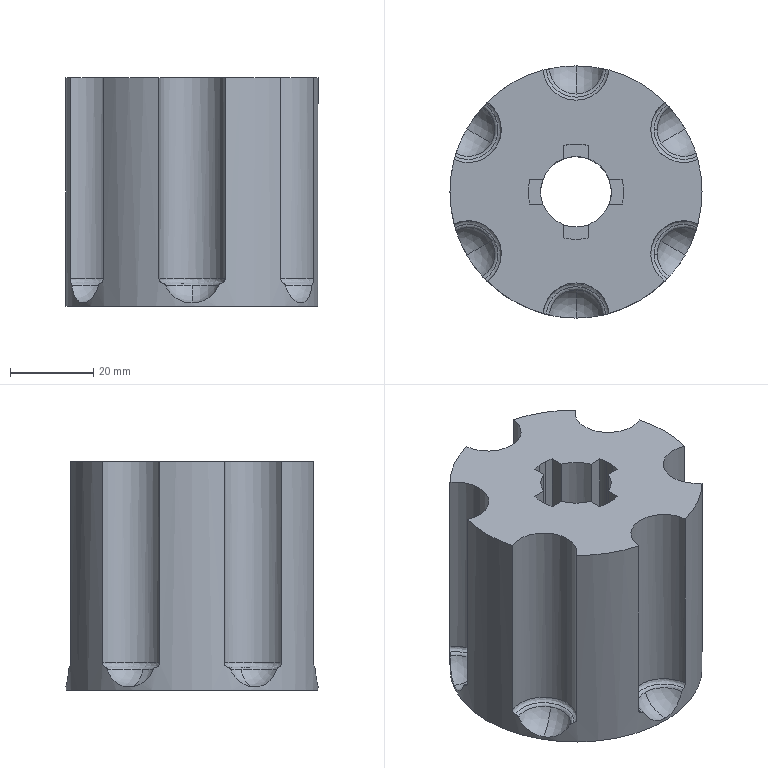Part | NX | features EXTRUDE 2, BREP 1, DATUM_CSYS 1, INTERSECT 1, LINKED_BODY 1, LINKED_FACE 1, SKETCH 1, UNITE 1 | 1 solid | 98 faces | box 60.7 x 60.7 x 55 mm | volume 113119 mm3 | cylinder 42 | plane 30 | sphere 12 | torus 8 | spline 6 | commonest cylinder face diameters 20 x24 16 x8 23 x8 17 x1 60.7 x1